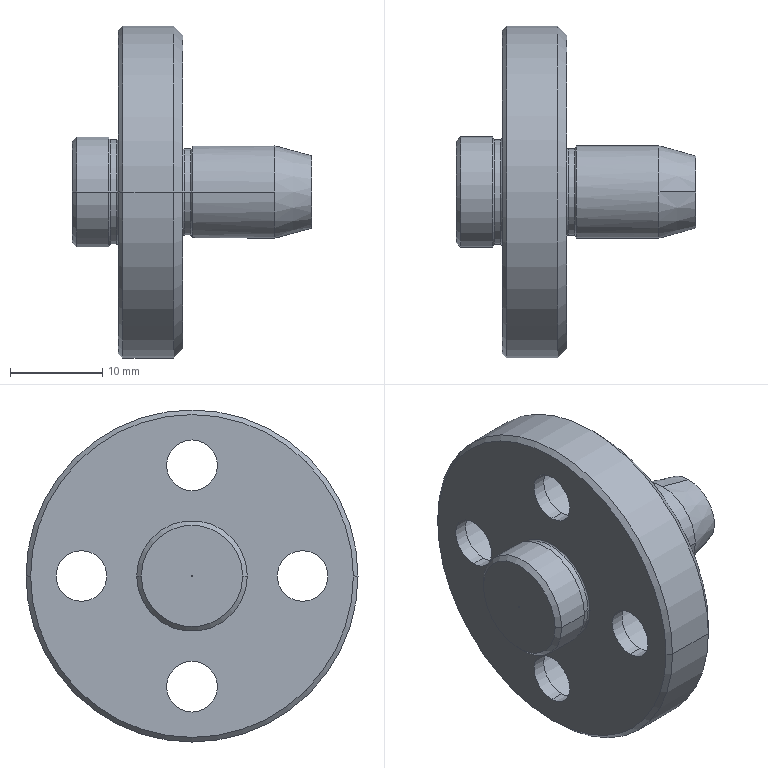Part | STEP file | MISUMI_MASAA12-P10.00-B10.0-T7.0_Locating pin | 1 solid | 56 faces | box 26 x 36 x 36 mm | volume 6932 mm3 | cylinder 26 | cone 12 | plane 10 | torus 8 | commonest cylinder face diameters 5.5 x8 9.5 x8 9.4 x2 10 x2 11.4 x2 12 x2
STEP:
#1=CARTESIAN_POINT('',(25.9,0.,0.));
#2=VERTEX_POINT('',#1);
#3=CARTESIAN_POINT('',(26.,0.,-0.1));
#4=VERTEX_POINT('',#3);
#5=CARTESIAN_POINT('',(26.,0.,-0.1));
#6=DIRECTION('',(0.7071,0.,-0.7071));
#7=VECTOR('',#6,1000.);
#8=LINE('',#5,#7);
#9=EDGE_CURVE('',#2,#4,#8,.T.);
#10=ORIENTED_EDGE('',*,*,#9,.F.);
#11=CARTESIAN_POINT('',(26.,0.,0.1));
#12=VERTEX_POINT('',#11);
#13=CARTESIAN_POINT('',(26.,0.,0.1));
#14=DIRECTION('',(0.7071,0.,0.7071));
#15=VECTOR('',#14,1000.);
#16=LINE('',#13,#15);
#17=EDGE_CURVE('',#2,#12,#16,.T.);
#18=ORIENTED_EDGE('',*,*,#17,.T.);
#19=CARTESIAN_POINT('',(26.,0.,0.));
#20=DIRECTION('',(-1.,0.,0.));
#21=DIRECTION('',(0.,0.,1.));
#22=AXIS2_PLACEMENT_3D('',#19,#20,#21);
#23=CIRCLE('',#22,0.1);
#24=EDGE_CURVE('',#4,#12,#23,.T.);
#25=ORIENTED_EDGE('',*,*,#24,.F.);
#26=EDGE_LOOP('',(#10,#18,#25));
#27=FACE_OUTER_BOUND('',#26,.T.);
#28=CARTESIAN_POINT('',(26.,0.,0.));
#29=DIRECTION('',(1.,0.,0.));
#30=DIRECTION('',(0.,0.,-1.));
#31=AXIS2_PLACEMENT_3D('',#28,#29,#30);
#32=CONICAL_SURFACE('',#31,0.1,0.7854);
#33=ADVANCED_FACE('',(#27),#32,.F.);
#34=CARTESIAN_POINT('',(26.,0.,3.928));
#35=VERTEX_POINT('',#34);
#36=CARTESIAN_POINT('',(26.,0.,-3.928));
#37=VERTEX_POINT('',#36);
#38=CARTESIAN_POINT('',(26.,0.,0.));
#39=DIRECTION('',(-1.,0.,0.));
#40=DIRECTION('',(0.,0.,1.));
#41=AXIS2_PLACEMENT_3D('',#38,#39,#40);
#42=CIRCLE('',#41,3.928);
#43=EDGE_CURVE('',#35,#37,#42,.T.);
#44=ORIENTED_EDGE('',*,*,#43,.T.);
#45=CARTESIAN_POINT('',(22.,0.,-5.));
#46=VERTEX_POINT('',#45);
#47=CARTESIAN_POINT('',(26.,0.,-3.928));
#48=DIRECTION('',(-0.9659,0.,-0.2588));
#49=VECTOR('',#48,1000.);
#50=LINE('',#47,#49);
#51=EDGE_CURVE('',#37,#46,#50,.T.);
#52=ORIENTED_EDGE('',*,*,#51,.T.);
#53=CARTESIAN_POINT('',(22.,5.,0.));
#54=VERTEX_POINT('',#53);
#55=CARTESIAN_POINT('',(22.,0.,0.));
#56=DIRECTION('',(-1.,0.,0.));
#57=DIRECTION('',(0.,0.,1.));
#58=AXIS2_PLACEMENT_3D('',#55,#56,#57);
#59=CIRCLE('',#58,5.);
#60=EDGE_CURVE('',#54,#46,#59,.T.);
#61=ORIENTED_EDGE('',*,*,#60,.F.);
#62=CARTESIAN_POINT('',(22.,0.,5.));
#63=VERTEX_POINT('',#62);
#64=CARTESIAN_POINT('',(22.,0.,0.));
#65=DIRECTION('',(-1.,0.,0.));
#66=DIRECTION('',(0.,0.,1.));
#67=AXIS2_PLACEMENT_3D('',#64,#65,#66);
#68=CIRCLE('',#67,5.);
#69=EDGE_CURVE('',#63,#54,#68,.T.);
#70=ORIENTED_EDGE('',*,*,#69,.F.);
#71=CARTESIAN_POINT('',(26.,0.,3.928));
#72=DIRECTION('',(-0.9659,0.,0.2588));
#73=VECTOR('',#72,1000.);
#74=LINE('',#71,#73);
#75=EDGE_CURVE('',#35,#63,#74,.T.);
#76=ORIENTED_EDGE('',*,*,#75,.F.);
#77=EDGE_LOOP('',(#44,#52,#61,#70,#76));
#78=FACE_OUTER_BOUND('',#77,.T.);
#79=CARTESIAN_POINT('',(26.,0.,0.));
#80=DIRECTION('',(-1.,0.,0.));
#81=DIRECTION('',(0.,0.,1.));
#82=AXIS2_PLACEMENT_3D('',#79,#80,#81);
#83=CONICAL_SURFACE('',#82,3.928,0.2618);
#84=ADVANCED_FACE('',(#78),#83,.T.);
#85=CARTESIAN_POINT('',(12.,17.,0.));
#86=VERTEX_POINT('',#85);
#87=CARTESIAN_POINT('',(12.,-17.,0.));
#88=VERTEX_POINT('',#87);
#89=CARTESIAN_POINT('',(12.,0.,0.));
#90=DIRECTION('',(1.,0.,0.));
#91=DIRECTION('',(0.,-1.,0.));
#92=AXIS2_PLACEMENT_3D('',#89,#90,#91);
#93=CIRCLE('',#92,17.);
#94=EDGE_CURVE('',#86,#88,#93,.T.);
#95=ORIENTED_EDGE('',*,*,#94,.F.);
#96=CARTESIAN_POINT('',(11.,18.,0.));
#97=VERTEX_POINT('',#96);
#98=CARTESIAN_POINT('',(11.,18.,0.));
#99=DIRECTION('',(-0.7071,0.7071,0.));
#100=VECTOR('',#99,1000.);
#101=LINE('',#98,#100);
#102=EDGE_CURVE('',#86,#97,#101,.T.);
#103=ORIENTED_EDGE('',*,*,#102,.T.);
#104=CARTESIAN_POINT('',(11.,-18.,0.));
#105=VERTEX_POINT('',#104);
#106=CARTESIAN_POINT('',(11.,0.,0.));
#107=DIRECTION('',(-1.,0.,0.));
#108=DIRECTION('',(0.,-1.,0.));
#109=AXIS2_PLACEMENT_3D('',#106,#107,#108);
#110=CIRCLE('',#109,18.);
#111=EDGE_CURVE('',#105,#97,#110,.T.);
#112=ORIENTED_EDGE('',*,*,#111,.F.);
#113=CARTESIAN_POINT('',(11.,-18.,0.));
#114=DIRECTION('',(-0.7071,-0.7071,0.));
#115=VECTOR('',#114,1000.);
#116=LINE('',#113,#115);
#117=EDGE_CURVE('',#88,#105,#116,.T.);
#118=ORIENTED_EDGE('',*,*,#117,.F.);
#119=EDGE_LOOP('',(#95,#103,#112,#118));
#120=FACE_OUTER_BOUND('',#119,.T.);
#121=CARTESIAN_POINT('',(11.,0.,0.));
#122=DIRECTION('',(-1.,0.,0.));
#123=DIRECTION('',(0.,-1.,0.));
#124=AXIS2_PLACEMENT_3D('',#121,#122,#123);
#125=CONICAL_SURFACE('',#124,18.,0.7854);
#126=ADVANCED_FACE('',(#120),#125,.T.);
#127=CARTESIAN_POINT('',(5.,-17.5,0.));
#128=VERTEX_POINT('',#127);
#129=CARTESIAN_POINT('',(5.,17.5,0.));
#130=VERTEX_POINT('',#129);
#131=CARTESIAN_POINT('',(5.,0.,0.));
#132=DIRECTION('',(-1.,0.,0.));
#133=DIRECTION('',(0.,1.,0.));
#134=AXIS2_PLACEMENT_3D('',#131,#132,#133);
#135=CIRCLE('',#134,17.5);
#136=EDGE_CURVE('',#128,#130,#135,.T.);
#137=ORIENTED_EDGE('',*,*,#136,.F.);
#138=CARTESIAN_POINT('',(5.5,-18.,0.));
#139=VERTEX_POINT('',#138);
#140=CARTESIAN_POINT('',(5.,-17.5,0.));
#141=DIRECTION('',(0.7071,-0.7071,0.));
#142=VECTOR('',#141,1000.);
#143=LINE('',#140,#142);
#144=EDGE_CURVE('',#128,#139,#143,.T.);
#145=ORIENTED_EDGE('',*,*,#144,.T.);
#146=CARTESIAN_POINT('',(5.5,18.,0.));
#147=VERTEX_POINT('',#146);
#148=CARTESIAN_POINT('',(5.5,0.,0.));
#149=DIRECTION('',(1.,0.,0.));
#150=DIRECTION('',(0.,1.,0.));
#151=AXIS2_PLACEMENT_3D('',#148,#149,#150);
#152=CIRCLE('',#151,18.);
#153=EDGE_CURVE('',#147,#139,#152,.T.);
#154=ORIENTED_EDGE('',*,*,#153,.F.);
#155=CARTESIAN_POINT('',(5.,17.5,0.));
#156=DIRECTION('',(0.7071,0.7071,0.));
#157=VECTOR('',#156,1000.);
#158=LINE('',#155,#157);
#159=EDGE_CURVE('',#130,#147,#158,.T.);
#160=ORIENTED_EDGE('',*,*,#159,.F.);
#161=EDGE_LOOP('',(#137,#145,#154,#160));
#162=FACE_OUTER_BOUND('',#161,.T.);
#163=CARTESIAN_POINT('',(5.,0.,0.));
#164=DIRECTION('',(1.,0.,0.));
#165=DIRECTION('',(0.,1.,0.));
#166=AXIS2_PLACEMENT_3D('',#163,#164,#165);
#167=CONICAL_SURFACE('',#166,17.5,0.7854);
#168=ADVANCED_FACE('',(#162),#167,.T.);
#169=CARTESIAN_POINT('',(12.,4.85,0.));
#170=VERTEX_POINT('',#169);
#171=CARTESIAN_POINT('',(12.,-4.85,0.));
#172=VERTEX_POINT('',#171);
#173=CARTESIAN_POINT('',(12.,0.,0.));
#174=DIRECTION('',(-1.,0.,0.));
#175=DIRECTION('',(0.,-1.,0.));
#176=AXIS2_PLACEMENT_3D('',#173,#174,#175);
#177=CIRCLE('',#176,4.85);
#178=EDGE_CURVE('',#170,#172,#177,.T.);
#179=ORIENTED_EDGE('',*,*,#178,.F.);
#180=CARTESIAN_POINT('',(12.15,4.7,0.));
#181=VERTEX_POINT('',#180);
#182=CARTESIAN_POINT('',(12.15,4.85,0.));
#183=DIRECTION('',(0.,0.,1.));
#184=DIRECTION('',(0.,-1.,0.));
#185=AXIS2_PLACEMENT_3D('',#182,#183,#184);
#186=CIRCLE('',#185,0.15);
#187=EDGE_CURVE('',#170,#181,#186,.T.);
#188=ORIENTED_EDGE('',*,*,#187,.T.);
#189=CARTESIAN_POINT('',(12.15,-4.7,0.));
#190=VERTEX_POINT('',#189);
#191=CARTESIAN_POINT('',(12.15,0.,0.));
#192=DIRECTION('',(1.,0.,0.));
#193=DIRECTION('',(0.,-1.,0.));
#194=AXIS2_PLACEMENT_3D('',#191,#192,#193);
#195=CIRCLE('',#194,4.7);
#196=EDGE_CURVE('',#190,#181,#195,.T.);
#197=ORIENTED_EDGE('',*,*,#196,.F.);
#198=CARTESIAN_POINT('',(12.15,-4.85,0.));
#199=DIRECTION('',(0.,0.,-1.));
#200=DIRECTION('',(-1.,0.,0.));
#201=AXIS2_PLACEMENT_3D('',#198,#199,#200);
#202=CIRCLE('',#201,0.15);
#203=EDGE_CURVE('',#172,#190,#202,.T.);
#204=ORIENTED_EDGE('',*,*,#203,.F.);
#205=EDGE_LOOP('',(#179,#188,#197,#204));
#206=FACE_OUTER_BOUND('',#205,.T.);
#207=CARTESIAN_POINT('',(12.15,0.,0.));
#208=DIRECTION('',(-1.,0.,0.));
#209=DIRECTION('',(0.,-1.,0.));
#210=AXIS2_PLACEMENT_3D('',#207,#208,#209);
#211=TOROIDAL_SURFACE('',#210,4.85,0.15);
#212=ADVANCED_FACE('',(#206),#211,.F.);
#213=CARTESIAN_POINT('',(13.,-4.85,0.));
#214=VERTEX_POINT('',#213);
#215=CARTESIAN_POINT('',(13.,4.85,0.));
#216=VERTEX_POINT('',#215);
#217=CARTESIAN_POINT('',(13.,0.,0.));
#218=DIRECTION('',(1.,0.,0.));
#219=DIRECTION('',(0.,1.,0.));
#220=AXIS2_PLACEMENT_3D('',#217,#218,#219);
#221=CIRCLE('',#220,4.85);
#222=EDGE_CURVE('',#214,#216,#221,.T.);
#223=ORIENTED_EDGE('',*,*,#222,.F.);
#224=CARTESIAN_POINT('',(12.85,-4.7,0.));
#225=VERTEX_POINT('',#224);
#226=CARTESIAN_POINT('',(12.85,-4.85,0.));
#227=DIRECTION('',(0.,0.,1.));
#228=DIRECTION('',(0.,-1.,0.));
#229=AXIS2_PLACEMENT_3D('',#226,#227,#228);
#230=CIRCLE('',#229,0.15);
#231=EDGE_CURVE('',#214,#225,#230,.T.);
#232=ORIENTED_EDGE('',*,*,#231,.T.);
#233=CARTESIAN_POINT('',(12.85,4.7,0.));
#234=VERTEX_POINT('',#233);
#235=CARTESIAN_POINT('',(12.85,0.,0.));
#236=DIRECTION('',(-1.,0.,0.));
#237=DIRECTION('',(0.,1.,0.));
#238=AXIS2_PLACEMENT_3D('',#235,#236,#237);
#239=CIRCLE('',#238,4.7);
#240=EDGE_CURVE('',#234,#225,#239,.T.);
#241=ORIENTED_EDGE('',*,*,#240,.F.);
#242=CARTESIAN_POINT('',(12.85,4.85,0.));
#243=DIRECTION('',(0.,0.,-1.));
#244=DIRECTION('',(-1.,0.,0.));
#245=AXIS2_PLACEMENT_3D('',#242,#243,#244);
#246=CIRCLE('',#245,0.15);
#247=EDGE_CURVE('',#216,#234,#246,.T.);
#248=ORIENTED_EDGE('',*,*,#247,.F.);
#249=EDGE_LOOP('',(#223,#232,#241,#248));
#250=FACE_OUTER_BOUND('',#249,.T.);
#251=CARTESIAN_POINT('',(12.85,0.,0.));
#252=DIRECTION('',(1.,0.,0.));
#253=DIRECTION('',(0.,1.,0.));
#254=AXIS2_PLACEMENT_3D('',#251,#252,#253);
#255=TOROIDAL_SURFACE('',#254,4.85,0.15);
#256=ADVANCED_FACE('',(#250),#255,.F.);
#257=CARTESIAN_POINT('',(5.,-5.85,0.));
#258=VERTEX_POINT('',#257);
#259=CARTESIAN_POINT('',(5.,5.85,0.));
#260=VERTEX_POINT('',#259);
#261=CARTESIAN_POINT('',(5.,0.,0.));
#262=DIRECTION('',(1.,0.,0.));
#263=DIRECTION('',(0.,1.,0.));
#264=AXIS2_PLACEMENT_3D('',#261,#262,#263);
#265=CIRCLE('',#264,5.85);
#266=EDGE_CURVE('',#258,#260,#265,.T.);
#267=ORIENTED_EDGE('',*,*,#266,.F.);
#268=CARTESIAN_POINT('',(4.85,-5.7,0.));
#269=VERTEX_POINT('',#268);
#270=CARTESIAN_POINT('',(4.85,-5.85,0.));
#271=DIRECTION('',(0.,0.,1.));
#272=DIRECTION('',(0.,-1.,0.));
#273=AXIS2_PLACEMENT_3D('',#270,#271,#272);
#274=CIRCLE('',#273,0.15);
#275=EDGE_CURVE('',#258,#269,#274,.T.);
#276=ORIENTED_EDGE('',*,*,#275,.T.);
#277=CARTESIAN_POINT('',(4.85,5.7,0.));
#278=VERTEX_POINT('',#277);
#279=CARTESIAN_POINT('',(4.85,0.,0.));
#280=DIRECTION('',(-1.,0.,0.));
#281=DIRECTION('',(0.,1.,0.));
#282=AXIS2_PLACEMENT_3D('',#279,#280,#281);
#283=CIRCLE('',#282,5.7);
#284=EDGE_CURVE('',#278,#269,#283,.T.);
#285=ORIENTED_EDGE('',*,*,#284,.F.);
#286=CARTESIAN_POINT('',(4.85,5.85,0.));
#287=DIRECTION('',(0.,0.,-1.));
#288=DIRECTION('',(-1.,0.,0.));
#289=AXIS2_PLACEMENT_3D('',#286,#287,#288);
#290=CIRCLE('',#289,0.15);
#291=EDGE_CURVE('',#260,#278,#290,.T.);
#292=ORIENTED_EDGE('',*,*,#291,.F.);
#293=EDGE_LOOP('',(#267,#276,#285,#292));
#294=FACE_OUTER_BOUND('',#293,.T.);
#295=CARTESIAN_POINT('',(4.85,0.,0.));
#296=DIRECTION('',(1.,0.,0.));
#297=DIRECTION('',(0.,1.,0.));
#298=AXIS2_PLACEMENT_3D('',#295,#296,#297);
#299=TOROIDAL_SURFACE('',#298,5.85,0.15);
#300=ADVANCED_FACE('',(#294),#299,.F.);
#301=CARTESIAN_POINT('',(4.,5.85,0.));
#302=VERTEX_POINT('',#301);
#303=CARTESIAN_POINT('',(4.,-5.85,0.));
#304=VERTEX_POINT('',#303);
#305=CARTESIAN_POINT('',(4.,0.,0.));
#306=DIRECTION('',(-1.,0.,0.));
#307=DIRECTION('',(0.,-1.,0.));
#308=AXIS2_PLACEMENT_3D('',#305,#306,#307);
#309=CIRCLE('',#308,5.85);
#310=EDGE_CURVE('',#302,#304,#309,.T.);
#311=ORIENTED_EDGE('',*,*,#310,.F.);
#312=CARTESIAN_POINT('',(4.15,5.7,0.));
#313=VERTEX_POINT('',#312);
#314=CARTESIAN_POINT('',(4.15,5.85,0.));
#315=DIRECTION('',(0.,0.,1.));
#316=DIRECTION('',(0.,-1.,0.));
#317=AXIS2_PLACEMENT_3D('',#314,#315,#316);
#318=CIRCLE('',#317,0.15);
#319=EDGE_CURVE('',#302,#313,#318,.T.);
#320=ORIENTED_EDGE('',*,*,#319,.T.);
#321=CARTESIAN_POINT('',(4.15,-5.7,0.));
#322=VERTEX_POINT('',#321);
#323=CARTESIAN_POINT('',(4.15,0.,0.));
#324=DIRECTION('',(1.,0.,0.));
#325=DIRECTION('',(0.,-1.,0.));
#326=AXIS2_PLACEMENT_3D('',#323,#324,#325);
#327=CIRCLE('',#326,5.7);
#328=EDGE_CURVE('',#322,#313,#327,.T.);
#329=ORIENTED_EDGE('',*,*,#328,.F.);
#330=CARTESIAN_POINT('',(4.15,-5.85,0.));
#331=DIRECTION('',(0.,0.,-1.));
#332=DIRECTION('',(-1.,0.,0.));
#333=AXIS2_PLACEMENT_3D('',#330,#331,#332);
#334=CIRCLE('',#333,0.15);
#335=EDGE_CURVE('',#304,#322,#334,.T.);
#336=ORIENTED_EDGE('',*,*,#335,.F.);
#337=EDGE_LOOP('',(#311,#320,#329,#336));
#338=FACE_OUTER_BOUND('',#337,.T.);
#339=CARTESIAN_POINT('',(4.15,0.,0.));
#340=DIRECTION('',(-1.,0.,0.));
#341=DIRECTION('',(0.,-1.,0.));
#342=AXIS2_PLACEMENT_3D('',#339,#340,#341);
#343=TOROIDAL_SURFACE('',#342,5.85,0.15);
#344=ADVANCED_FACE('',(#338),#343,.F.);
#345=CARTESIAN_POINT('',(0.,-5.5,0.));
#346=VERTEX_POINT('',#345);
#347=CARTESIAN_POINT('',(0.,5.5,0.));
#348=VERTEX_POINT('',#347);
#349=CARTESIAN_POINT('',(0.,0.,0.));
#350=DIRECTION('',(-1.,0.,0.));
#351=DIRECTION('',(0.,1.,0.));
#352=AXIS2_PLACEMENT_3D('',#349,#350,#351);
#353=CIRCLE('',#352,5.5);
#354=EDGE_CURVE('',#346,#348,#353,.T.);
#355=ORIENTED_EDGE('',*,*,#354,.F.);
#356=CARTESIAN_POINT('',(0.5,-6.,0.));
#357=VERTEX_POINT('',#356);
#358=CARTESIAN_POINT('',(0.,-5.5,0.));
#359=DIRECTION('',(0.7071,-0.7071,0.));
#360=VECTOR('',#359,1000.);
#361=LINE('',#358,#360);
#362=EDGE_CURVE('',#346,#357,#361,.T.);
#363=ORIENTED_EDGE('',*,*,#362,.T.);
#364=CARTESIAN_POINT('',(0.5,6.,0.));
#365=VERTEX_POINT('',#364);
#366=CARTESIAN_POINT('',(0.5,0.,0.));
#367=DIRECTION('',(1.,0.,0.));
#368=DIRECTION('',(0.,1.,0.));
#369=AXIS2_PLACEMENT_3D('',#366,#367,#368);
#370=CIRCLE('',#369,6.);
#371=EDGE_CURVE('',#365,#357,#370,.T.);
#372=ORIENTED_EDGE('',*,*,#371,.F.);
#373=CARTESIAN_POINT('',(0.,5.5,0.));
#374=DIRECTION('',(0.7071,0.7071,0.));
#375=VECTOR('',#374,1000.);
#376=LINE('',#373,#375);
#377=EDGE_CURVE('',#348,#365,#376,.T.);
#378=ORIENTED_EDGE('',*,*,#377,.F.);
#379=EDGE_LOOP('',(#355,#363,#372,#378));
#380=FACE_OUTER_BOUND('',#379,.T.);
#381=CARTESIAN_POINT('',(0.,0.,0.));
#382=DIRECTION('',(1.,0.,0.));
#383=DIRECTION('',(0.,1.,0.));
#384=AXIS2_PLACEMENT_3D('',#381,#382,#383);
#385=CONICAL_SURFACE('',#384,5.5,0.7854);
#386=ADVANCED_FACE('',(#380),#385,.T.);
#387=CARTESIAN_POINT('',(6.5,12.,4.75));
#388=VERTEX_POINT('',#387);
#389=CARTESIAN_POINT('',(6.5,12.,-4.75));
#390=VERTEX_POINT('',#389);
#391=CARTESIAN_POINT('',(6.5,12.,0.));
#392=DIRECTION('',(1.,0.,0.));
#393=DIRECTION('',(0.,0.,-1.));
#394=AXIS2_PLACEMENT_3D('',#391,#392,#393);
#395=CIRCLE('',#394,4.75);
#396=EDGE_CURVE('',#388,#390,#395,.T.);
#397=ORIENTED_EDGE('',*,*,#396,.F.);
#398=CARTESIAN_POINT('',(12.,12.,4.75));
#399=VERTEX_POINT('',#398);
#400=CARTESIAN_POINT('',(12.,12.,4.75));
#401=DIRECTION('',(1.,0.,0.));
#402=VECTOR('',#401,1000.);
#403=LINE('',#400,#402);
#404=EDGE_CURVE('',#388,#399,#403,.T.);
#405=ORIENTED_EDGE('',*,*,#404,.T.);
#406=CARTESIAN_POINT('',(12.,12.,-4.75));
#407=VERTEX_POINT('',#406);
#408=CARTESIAN_POINT('',(12.,12.,0.));
#409=DIRECTION('',(1.,0.,0.));
#410=DIRECTION('',(0.,0.,-1.));
#411=AXIS2_PLACEMENT_3D('',#408,#409,#410);
#412=CIRCLE('',#411,4.75);
#413=EDGE_CURVE('',#399,#407,#412,.T.);
#414=ORIENTED_EDGE('',*,*,#413,.T.);
#415=CARTESIAN_POINT('',(12.,12.,-4.75));
#416=DIRECTION('',(1.,0.,0.));
#417=VECTOR('',#416,1000.);
#418=LINE('',#415,#417);
#419=EDGE_CURVE('',#390,#407,#418,.T.);
#420=ORIENTED_EDGE('',*,*,#419,.F.);
#421=EDGE_LOOP('',(#397,#405,#414,#420));
#422=FACE_OUTER_BOUND('',#421,.T.);
#423=CARTESIAN_POINT('',(12.,12.,0.));
#424=DIRECTION('',(1.,0.,0.));
#425=DIRECTION('',(0.,0.,-1.));
#426=AXIS2_PLACEMENT_3D('',#423,#424,#425);
#427=CYLINDRICAL_SURFACE('',#426,4.75);
#428=ADVANCED_FACE('',(#422),#427,.F.);
#429=CARTESIAN_POINT('',(5.,12.,2.75));
#430=VERTEX_POINT('',#429);
#431=CARTESIAN_POINT('',(5.,12.,-2.75));
#432=VERTEX_POINT('',#431);
#433=CARTESIAN_POINT('',(5.,12.,0.));
#434=DIRECTION('',(1.,0.,0.));
#435=DIRECTION('',(0.,1.,0.));
#436=AXIS2_PLACEMENT_3D('',#433,#434,#435);
#437=CIRCLE('',#436,2.75);
#438=EDGE_CURVE('',#430,#432,#437,.T.);
#439=ORIENTED_EDGE('',*,*,#438,.F.);
#440=CARTESIAN_POINT('',(6.5,12.,2.75));
#441=VERTEX_POINT('',#440);
#442=CARTESIAN_POINT('',(12.,12.,2.75));
#443=DIRECTION('',(1.,0.,0.));
#444=VECTOR('',#443,1000.);
#445=LINE('',#442,#444);
#446=EDGE_CURVE('',#430,#441,#445,.T.);
#447=ORIENTED_EDGE('',*,*,#446,.T.);
#448=CARTESIAN_POINT('',(6.5,12.,-2.75));
#449=VERTEX_POINT('',#448);
#450=CARTESIAN_POINT('',(6.5,12.,0.));
#451=DIRECTION('',(1.,0.,0.));
#452=DIRECTION('',(0.,0.,-1.));
#453=AXIS2_PLACEMENT_3D('',#450,#451,#452);
#454=CIRCLE('',#453,2.75);
#455=EDGE_CURVE('',#441,#449,#454,.T.);
#456=ORIENTED_EDGE('',*,*,#455,.T.);
#457=CARTESIAN_POINT('',(12.,12.,-2.75));
#458=DIRECTION('',(1.,0.,0.));
#459=VECTOR('',#458,1000.);
#460=LINE('',#457,#459);
#461=EDGE_CURVE('',#432,#449,#460,.T.);
#462=ORIENTED_EDGE('',*,*,#461,.F.);
#463=EDGE_LOOP('',(#439,#447,#456,#462));
#464=FACE_OUTER_BOUND('',#463,.T.);
#465=CARTESIAN_POINT('',(12.,12.,0.));
#466=DIRECTION('',(1.,0.,0.));
#467=DIRECTION('',(0.,0.,-1.));
#468=AXIS2_PLACEMENT_3D('',#465,#466,#467);
#469=CYLINDRICAL_SURFACE('',#468,2.75);
#470=ADVANCED_FACE('',(#464),#469,.F.);
#471=CARTESIAN_POINT('',(6.5,0.,16.75));
#472=VERTEX_POINT('',#471);
#473=CARTESIAN_POINT('',(6.5,0.,7.25));
#474=VERTEX_POINT('',#473);
#475=CARTESIAN_POINT('',(6.5,0.,12.));
#476=DIRECTION('',(1.,0.,0.));
#477=DIRECTION('',(0.,0.,-1.));
#478=AXIS2_PLACEMENT_3D('',#475,#476,#477);
#479=CIRCLE('',#478,4.75);
#480=EDGE_CURVE('',#472,#474,#479,.T.);
#481=ORIENTED_EDGE('',*,*,#480,.F.);
#482=CARTESIAN_POINT('',(12.,0.,16.75));
#483=VERTEX_POINT('',#482);
#484=CARTESIAN_POINT('',(12.,0.,16.75));
#485=DIRECTION('',(1.,0.,0.));
#486=VECTOR('',#485,1000.);
#487=LINE('',#484,#486);
#488=EDGE_CURVE('',#472,#483,#487,.T.);
#489=ORIENTED_EDGE('',*,*,#488,.T.);
#490=CARTESIAN_POINT('',(12.,0.,7.25));
#491=VERTEX_POINT('',#490);
#492=CARTESIAN_POINT('',(12.,0.,12.));
#493=DIRECTION('',(1.,0.,0.));
#494=DIRECTION('',(0.,0.,-1.));
#495=AXIS2_PLACEMENT_3D('',#492,#493,#494);
#496=CIRCLE('',#495,4.75);
#497=EDGE_CURVE('',#483,#491,#496,.T.);
#498=ORIENTED_EDGE('',*,*,#497,.T.);
#499=CARTESIAN_POINT('',(12.,0.,7.25));
#500=DIRECTION('',(1.,0.,0.));
#501=VECTOR('',#500,1000.);
#502=LINE('',#499,#501);
#503=EDGE_CURVE('',#474,#491,#502,.T.);
#504=ORIENTED_EDGE('',*,*,#503,.F.);
#505=EDGE_LOOP('',(#481,#489,#498,#504));
#506=FACE_OUTER_BOUND('',#505,.T.);
#507=CARTESIAN_POINT('',(12.,0.,12.));
#508=DIRECTION('',(1.,0.,0.));
#509=DIRECTION('',(0.,0.,-1.));
#510=AXIS2_PLACEMENT_3D('',#507,#508,#509);
#511=CYLINDRICAL_SURFACE('',#510,4.75);
#512=ADVANCED_FACE('',(#506),#511,.F.);
#513=CARTESIAN_POINT('',(5.,0.,14.75));
#514=VERTEX_POINT('',#513);
#515=CARTESIAN_POINT('',(5.,0.,9.25));
#516=VERTEX_POINT('',#515);
#517=CARTESIAN_POINT('',(5.,0.,12.));
#518=DIRECTION('',(1.,0.,0.));
#519=DIRECTION('',(0.,1.,0.));
#520=AXIS2_PLACEMENT_3D('',#517,#518,#519);
#521=CIRCLE('',#520,2.75);
#522=EDGE_CURVE('',#514,#516,#521,.T.);
#523=ORIENTED_EDGE('',*,*,#522,.F.);
#524=CARTESIAN_POINT('',(6.5,0.,14.75));
#525=VERTEX_POINT('',#524);
#526=CARTESIAN_POINT('',(12.,0.,14.75));
#527=DIRECTION('',(1.,0.,0.));
#528=VECTOR('',#527,1000.);
#529=LINE('',#526,#528);
#530=EDGE_CURVE('',#514,#525,#529,.T.);
#531=ORIENTED_EDGE('',*,*,#530,.T.);
#532=CARTESIAN_POINT('',(6.5,0.,9.25));
#533=VERTEX_POINT('',#532);
#534=CARTESIAN_POINT('',(6.5,0.,12.));
#535=DIRECTION('',(1.,0.,0.));
#536=DIRECTION('',(0.,0.,-1.));
#537=AXIS2_PLACEMENT_3D('',#534,#535,#536);
#538=CIRCLE('',#537,2.75);
#539=EDGE_CURVE('',#525,#533,#538,.T.);
#540=ORIENTED_EDGE('',*,*,#539,.T.);
#541=CARTESIAN_POINT('',(12.,0.,9.25));
#542=DIRECTION('',(1.,0.,0.));
#543=VECTOR('',#542,1000.);
#544=LINE('',#541,#543);
#545=EDGE_CURVE('',#516,#533,#544,.T.);
#546=ORIENTED_EDGE('',*,*,#545,.F.);
#547=EDGE_LOOP('',(#523,#531,#540,#546));
#548=FACE_OUTER_BOUND('',#547,.T.);
#549=CARTESIAN_POINT('',(12.,0.,12.));
#550=DIRECTION('',(1.,0.,0.));
#551=DIRECTION('',(0.,0.,-1.));
#552=AXIS2_PLACEMENT_3D('',#549,#550,#551);
#553=CYLINDRICAL_SURFACE('',#552,2.75);
#554=ADVANCED_FACE('',(#548),#553,.F.);
#555=CARTESIAN_POINT('',(6.5,-12.,4.75));
#556=VERTEX_POINT('',#555);
#557=CARTESIAN_POINT('',(6.5,-12.,-4.75));
#558=VERTEX_POINT('',#557);
#559=CARTESIAN_POINT('',(6.5,-12.,0.));
#560=DIRECTION('',(1.,0.,0.));
#561=DIRECTION('',(0.,0.,-1.));
#562=AXIS2_PLACEMENT_3D('',#559,#560,#561);
#563=CIRCLE('',#562,4.75);
#564=EDGE_CURVE('',#556,#558,#563,.T.);
#565=ORIENTED_EDGE('',*,*,#564,.F.);
#566=CARTESIAN_POINT('',(12.,-12.,4.75));
#567=VERTEX_POINT('',#566);
#568=CARTESIAN_POINT('',(12.,-12.,4.75));
#569=DIRECTION('',(1.,0.,0.));
#570=VECTOR('',#569,1000.);
#571=LINE('',#568,#570);
#572=EDGE_CURVE('',#556,#567,#571,.T.);
#573=ORIENTED_EDGE('',*,*,#572,.T.);
#574=CARTESIAN_POINT('',(12.,-12.,-4.75));
#575=VERTEX_POINT('',#574);
#576=CARTESIAN_POINT('',(12.,-12.,0.));
#577=DIRECTION('',(1.,0.,0.));
#578=DIRECTION('',(0.,0.,-1.));
#579=AXIS2_PLACEMENT_3D('',#576,#577,#578);
#580=CIRCLE('',#579,4.75);
#581=EDGE_CURVE('',#567,#575,#580,.T.);
#582=ORIENTED_EDGE('',*,*,#581,.T.);
#583=CARTESIAN_POINT('',(12.,-12.,-4.75));
#584=DIRECTION('',(1.,0.,0.));
#585=VECTOR('',#584,1000.);
#586=LINE('',#583,#585);
#587=EDGE_CURVE('',#558,#575,#586,.T.);
#588=ORIENTED_EDGE('',*,*,#587,.F.);
#589=EDGE_LOOP('',(#565,#573,#582,#588));
#590=FACE_OUTER_BOUND('',#589,.T.);
#591=CARTESIAN_POINT('',(12.,-12.,0.));
#592=DIRECTION('',(1.,0.,0.));
#593=DIRECTION('',(0.,0.,-1.));
#594=AXIS2_PLACEMENT_3D('',#591,#592,#593);
#595=CYLINDRICAL_SURFACE('',#594,4.75);
#596=ADVANCED_FACE('',(#590),#595,.F.);
#597=CARTESIAN_POINT('',(5.,-12.,2.75));
#598=VERTEX_POINT('',#597);
#599=CARTESIAN_POINT('',(5.,-12.,-2.75));
#600=VERTEX_POINT('',#599);
#601=CARTESIAN_POINT('',(5.,-12.,0.));
#602=DIRECTION('',(1.,0.,0.));
#603=DIRECTION('',(0.,1.,0.));
#604=AXIS2_PLACEMENT_3D('',#601,#602,#603);
#605=CIRCLE('',#604,2.75);
#606=EDGE_CURVE('',#598,#600,#605,.T.);
#607=ORIENTED_EDGE('',*,*,#606,.F.);
#608=CARTESIAN_POINT('',(6.5,-12.,2.75));
#609=VERTEX_POINT('',#608);
#610=CARTESIAN_POINT('',(12.,-12.,2.75));
#611=DIRECTION('',(1.,0.,0.));
#612=VECTOR('',#611,1000.);
#613=LINE('',#610,#612);
#614=EDGE_CURVE('',#598,#609,#613,.T.);
#615=ORIENTED_EDGE('',*,*,#614,.T.);
#616=CARTESIAN_POINT('',(6.5,-12.,-2.75));
#617=VERTEX_POINT('',#616);
#618=CARTESIAN_POINT('',(6.5,-12.,0.));
#619=DIRECTION('',(1.,0.,0.));
#620=DIRECTION('',(0.,0.,-1.));
#621=AXIS2_PLACEMENT_3D('',#618,#619,#620);
#622=CIRCLE('',#621,2.75);
#623=EDGE_CURVE('',#609,#617,#622,.T.);
#624=ORIENTED_EDGE('',*,*,#623,.T.);
#625=CARTESIAN_POINT('',(12.,-12.,-2.75));
#626=DIRECTION('',(1.,0.,0.));
#627=VECTOR('',#626,1000.);
#628=LINE('',#625,#627);
#629=EDGE_CURVE('',#600,#617,#628,.T.);
#630=ORIENTED_EDGE('',*,*,#629,.F.);
#631=EDGE_LOOP('',(#607,#615,#624,#630));
#632=FACE_OUTER_BOUND('',#631,.T.);
#633=CARTESIAN_POINT('',(12.,-12.,0.));
#634=DIRECTION('',(1.,0.,0.));
#635=DIRECTION('',(0.,0.,-1.));
#636=AXIS2_PLACEMENT_3D('',#633,#634,#635);
#637=CYLINDRICAL_SURFACE('',#636,2.75);
#638=ADVANCED_FACE('',(#632),#637,.F.);
#639=CARTESIAN_POINT('',(6.5,0.,-7.25));
#640=VERTEX_POINT('',#639);
#641=CARTESIAN_POINT('',(6.5,0.,-16.75));
#642=VERTEX_POINT('',#641);
#643=CARTESIAN_POINT('',(6.5,0.,-12.));
#644=DIRECTION('',(1.,0.,0.));
#645=DIRECTION('',(0.,0.,-1.));
#646=AXIS2_PLACEMENT_3D('',#643,#644,#645);
#647=CIRCLE('',#646,4.75);
#648=EDGE_CURVE('',#640,#642,#647,.T.);
#649=ORIENTED_EDGE('',*,*,#648,.F.);
#650=CARTESIAN_POINT('',(12.,0.,-7.25));
#651=VERTEX_POINT('',#650);
#652=CARTESIAN_POINT('',(12.,0.,-7.25));
#653=DIRECTION('',(1.,0.,0.));
#654=VECTOR('',#653,1000.);
#655=LINE('',#652,#654);
#656=EDGE_CURVE('',#640,#651,#655,.T.);
#657=ORIENTED_EDGE('',*,*,#656,.T.);
#658=CARTESIAN_POINT('',(12.,0.,-16.75));
#659=VERTEX_POINT('',#658);
#660=CARTESIAN_POINT('',(12.,0.,-12.));
#661=DIRECTION('',(1.,0.,0.));
#662=DIRECTION('',(0.,0.,-1.));
#663=AXIS2_PLACEMENT_3D('',#660,#661,#662);
#664=CIRCLE('',#663,4.75);
#665=EDGE_CURVE('',#651,#659,#664,.T.);
#666=ORIENTED_EDGE('',*,*,#665,.T.);
#667=CARTESIAN_POINT('',(12.,0.,-16.75));
#668=DIRECTION('',(1.,0.,0.));
#669=VECTOR('',#668,1000.);
#670=LINE('',#667,#669);
#671=EDGE_CURVE('',#642,#659,#670,.T.);
#672=ORIENTED_EDGE('',*,*,#671,.F.);
#673=EDGE_LOOP('',(#649,#657,#666,#672));
#674=FACE_OUTER_BOUND('',#673,.T.);
#675=CARTESIAN_POINT('',(12.,0.,-12.));
#676=DIRECTION('',(1.,0.,0.));
#677=DIRECTION('',(0.,0.,-1.));
#678=AXIS2_PLACEMENT_3D('',#675,#676,#677);
#679=CYLINDRICAL_SURFACE('',#678,4.75);
#680=ADVANCED_FACE('',(#674),#679,.F.);
#681=CARTESIAN_POINT('',(5.,0.,-9.25));
#682=VERTEX_POINT('',#681);
#683=CARTESIAN_POINT('',(5.,0.,-14.75));
#684=VERTEX_POINT('',#683);
#685=CARTESIAN_POINT('',(5.,0.,-12.));
#686=DIRECTION('',(1.,0.,0.));
#687=DIRECTION('',(0.,1.,0.));
#688=AXIS2_PLACEMENT_3D('',#685,#686,#687);
#689=CIRCLE('',#688,2.75);
#690=EDGE_CURVE('',#682,#684,#689,.T.);
#691=ORIENTED_EDGE('',*,*,#690,.F.);
#692=CARTESIAN_POINT('',(6.5,0.,-9.25));
#693=VERTEX_POINT('',#692);
#694=CARTESIAN_POINT('',(12.,0.,-9.25));
#695=DIRECTION('',(1.,0.,0.));
#696=VECTOR('',#695,1000.);
#697=LINE('',#694,#696);
#698=EDGE_CURVE('',#682,#693,#697,.T.);
#699=ORIENTED_EDGE('',*,*,#698,.T.);
#700=CARTESIAN_POINT('',(6.5,0.,-14.75));
#701=VERTEX_POINT('',#700);
#702=CARTESIAN_POINT('',(6.5,0.,-12.));
#703=DIRECTION('',(1.,0.,0.));
#704=DIRECTION('',(0.,0.,-1.));
#705=AXIS2_PLACEMENT_3D('',#702,#703,#704);
#706=CIRCLE('',#705,2.75);
#707=EDGE_CURVE('',#693,#701,#706,.T.);
#708=ORIENTED_EDGE('',*,*,#707,.T.);
#709=CARTESIAN_POINT('',(12.,0.,-14.75));
#710=DIRECTION('',(1.,0.,0.));
#711=VECTOR('',#710,1000.);
#712=LINE('',#709,#711);
#713=EDGE_CURVE('',#684,#701,#712,.T.);
#714=ORIENTED_EDGE('',*,*,#713,.F.);
#715=EDGE_LOOP('',(#691,#699,#708,#714));
#716=FACE_OUTER_BOUND('',#715,.T.);
#717=CARTESIAN_POINT('',(12.,0.,-12.));
#718=DIRECTION('',(1.,0.,0.));
#719=DIRECTION('',(0.,0.,-1.));
#720=AXIS2_PLACEMENT_3D('',#717,#718,#719);
#721=CYLINDRICAL_SURFACE('',#720,2.75);
#722=ADVANCED_FACE('',(#716),#721,.F.);
#723=CARTESIAN_POINT('',(0.1,0.,0.));
#724=VERTEX_POINT('',#723);
#725=CARTESIAN_POINT('',(0.,0.,0.1));
#726=VERTEX_POINT('',#725);
#727=CARTESIAN_POINT('',(0.1,0.,0.));
#728=DIRECTION('',(-0.7071,0.,0.7071));
#729=VECTOR('',#728,1000.);
#730=LINE('',#727,#729);
#731=EDGE_CURVE('',#724,#726,#730,.T.);
#732=ORIENTED_EDGE('',*,*,#731,.F.);
#733=CARTESIAN_POINT('',(0.,0.,-0.1));
#734=VERTEX_POINT('',#733);
#735=CARTESIAN_POINT('',(0.1,0.,0.));
#736=DIRECTION('',(-0.7071,0.,-0.7071));
#737=VECTOR('',#736,1000.);
#738=LINE('',#735,#737);
#739=EDGE_CURVE('',#724,#734,#738,.T.);
#740=ORIENTED_EDGE('',*,*,#739,.T.);
#741=CARTESIAN_POINT('',(0.,0.,0.));
#742=DIRECTION('',(-1.,0.,0.));
#743=DIRECTION('',(0.,0.,1.));
#744=AXIS2_PLACEMENT_3D('',#741,#742,#743);
#745=CIRCLE('',#744,0.1);
#746=EDGE_CURVE('',#734,#726,#745,.T.);
#747=ORIENTED_EDGE('',*,*,#746,.T.);
#748=EDGE_LOOP('',(#732,#740,#747));
#749=FACE_OUTER_BOUND('',#748,.T.);
#750=CARTESIAN_POINT('',(-999.9,0.,0.));
#751=DIRECTION('',(-1.,0.,0.));
#752=DIRECTION('',(0.,0.,1.));
#753=AXIS2_PLACEMENT_3D('',#750,#751,#752);
#754=CONICAL_SURFACE('',#753,1000.,0.7854);
#755=ADVANCED_FACE('',(#749),#754,.F.);
#756=CARTESIAN_POINT('',(22.,-5.,0.));
#757=VERTEX_POINT('',#756);
#758=CARTESIAN_POINT('',(22.,0.,0.));
#759=DIRECTION('',(-1.,0.,0.));
#760=DIRECTION('',(0.,0.,1.));
#761=AXIS2_PLACEMENT_3D('',#758,#759,#760);
#762=CIRCLE('',#761,5.);
#763=EDGE_CURVE('',#757,#63,#762,.T.);
#764=ORIENTED_EDGE('',*,*,#763,.T.);
#765=ORIENTED_EDGE('',*,*,#69,.T.);
#766=CARTESIAN_POINT('',(13.,5.,0.));
#767=VERTEX_POINT('',#766);
#768=CARTESIAN_POINT('',(0.,5.,0.));
#769=DIRECTION('',(-1.,0.,0.));
#770=VECTOR('',#769,1000.);
#771=LINE('',#768,#770);
#772=EDGE_CURVE('',#54,#767,#771,.T.);
#773=ORIENTED_EDGE('',*,*,#772,.T.);
#774=CARTESIAN_POINT('',(13.,-5.,0.));
#775=VERTEX_POINT('',#774);
#776=CARTESIAN_POINT('',(13.,0.,0.));
#777=DIRECTION('',(-1.,0.,0.));
#778=DIRECTION('',(0.,-1.,0.));
#779=AXIS2_PLACEMENT_3D('',#776,#777,#778);
#780=CIRCLE('',#779,5.);
#781=EDGE_CURVE('',#775,#767,#780,.T.);
#782=ORIENTED_EDGE('',*,*,#781,.F.);
#783=CARTESIAN_POINT('',(0.,-5.,0.));
#784=DIRECTION('',(-1.,0.,0.));
#785=VECTOR('',#784,1000.);
#786=LINE('',#783,#785);
#787=EDGE_CURVE('',#757,#775,#786,.T.);
#788=ORIENTED_EDGE('',*,*,#787,.F.);
#789=EDGE_LOOP('',(#764,#765,#773,#782,#788));
#790=FACE_OUTER_BOUND('',#789,.T.);
#791=CARTESIAN_POINT('',(0.,0.,0.));
#792=DIRECTION('',(-1.,0.,0.));
#793=DIRECTION('',(0.,-1.,0.));
#794=AXIS2_PLACEMENT_3D('',#791,#792,#793);
#795=CYLINDRICAL_SURFACE('',#794,5.);
#796=ADVANCED_FACE('',(#790),#795,.T.);
#797=CARTESIAN_POINT('',(12.85,0.,0.));
#798=DIRECTION('',(-1.,0.,0.));
#799=DIRECTION('',(0.,1.,0.));
#800=AXIS2_PLACEMENT_3D('',#797,#798,#799);
#801=CIRCLE('',#800,4.7);
#802=EDGE_CURVE('',#225,#234,#801,.T.);
#803=ORIENTED_EDGE('',*,*,#802,.T.);
#804=CARTESIAN_POINT('',(0.,4.7,0.));
#805=DIRECTION('',(-1.,0.,0.));
#806=VECTOR('',#805,1000.);
#807=LINE('',#804,#806);
#808=EDGE_CURVE('',#234,#181,#807,.T.);
#809=ORIENTED_EDGE('',*,*,#808,.T.);
#810=CARTESIAN_POINT('',(12.15,0.,0.));
#811=DIRECTION('',(1.,0.,0.));
#812=DIRECTION('',(0.,-1.,0.));
#813=AXIS2_PLACEMENT_3D('',#810,#811,#812);
#814=CIRCLE('',#813,4.7);
#815=EDGE_CURVE('',#181,#190,#814,.T.);
#816=ORIENTED_EDGE('',*,*,#815,.T.);
#817=CARTESIAN_POINT('',(0.,-4.7,0.));
#818=DIRECTION('',(-1.,0.,0.));
#819=VECTOR('',#818,1000.);
#820=LINE('',#817,#819);
#821=EDGE_CURVE('',#225,#190,#820,.T.);
#822=ORIENTED_EDGE('',*,*,#821,.F.);
#823=EDGE_LOOP('',(#803,#809,#816,#822));
#824=FACE_OUTER_BOUND('',#823,.T.);
#825=CARTESIAN_POINT('',(0.,0.,0.));
#826=DIRECTION('',(-1.,0.,0.));
#827=DIRECTION('',(0.,-1.,0.));
#828=AXIS2_PLACEMENT_3D('',#825,#826,#827);
#829=CYLINDRICAL_SURFACE('',#828,4.7);
#830=ADVANCED_FACE('',(#824),#829,.T.);
#831=ORIENTED_EDGE('',*,*,#111,.T.);
#832=CARTESIAN_POINT('',(0.,18.,0.));
#833=DIRECTION('',(-1.,0.,0.));
#834=VECTOR('',#833,1000.);
#835=LINE('',#832,#834);
#836=EDGE_CURVE('',#97,#147,#835,.T.);
#837=ORIENTED_EDGE('',*,*,#836,.T.);
#838=ORIENTED_EDGE('',*,*,#153,.T.);
#839=CARTESIAN_POINT('',(0.,-18.,0.));
#840=DIRECTION('',(-1.,0.,0.));
#841=VECTOR('',#840,1000.);
#842=LINE('',#839,#841);
#843=EDGE_CURVE('',#105,#139,#842,.T.);
#844=ORIENTED_EDGE('',*,*,#843,.F.);
#845=EDGE_LOOP('',(#831,#837,#838,#844));
#846=FACE_OUTER_BOUND('',#845,.T.);
#847=CARTESIAN_POINT('',(0.,0.,0.));
#848=DIRECTION('',(-1.,0.,0.));
#849=DIRECTION('',(0.,-1.,0.));
#850=AXIS2_PLACEMENT_3D('',#847,#848,#849);
#851=CYLINDRICAL_SURFACE('',#850,18.);
#852=ADVANCED_FACE('',(#846),#851,.T.);
#853=CARTESIAN_POINT('',(4.85,0.,0.));
#854=DIRECTION('',(-1.,0.,0.));
#855=DIRECTION('',(0.,1.,0.));
#856=AXIS2_PLACEMENT_3D('',#853,#854,#855);
#857=CIRCLE('',#856,5.7);
#858=EDGE_CURVE('',#269,#278,#857,.T.);
#859=ORIENTED_EDGE('',*,*,#858,.T.);
#860=CARTESIAN_POINT('',(0.,5.7,0.));
#861=DIRECTION('',(-1.,0.,0.));
#862=VECTOR('',#861,1000.);
#863=LINE('',#860,#862);
#864=EDGE_CURVE('',#278,#313,#863,.T.);
#865=ORIENTED_EDGE('',*,*,#864,.T.);
#866=CARTESIAN_POINT('',(4.15,0.,0.));
#867=DIRECTION('',(1.,0.,0.));
#868=DIRECTION('',(0.,-1.,0.));
#869=AXIS2_PLACEMENT_3D('',#866,#867,#868);
#870=CIRCLE('',#869,5.7);
#871=EDGE_CURVE('',#313,#322,#870,.T.);
#872=ORIENTED_EDGE('',*,*,#871,.T.);
#873=CARTESIAN_POINT('',(0.,-5.7,0.));
#874=DIRECTION('',(-1.,0.,0.));
#875=VECTOR('',#874,1000.);
#876=LINE('',#873,#875);
#877=EDGE_CURVE('',#269,#322,#876,.T.);
#878=ORIENTED_EDGE('',*,*,#877,.F.);
#879=EDGE_LOOP('',(#859,#865,#872,#878));
#880=FACE_OUTER_BOUND('',#879,.T.);
#881=CARTESIAN_POINT('',(0.,0.,0.));
#882=DIRECTION('',(-1.,0.,0.));
#883=DIRECTION('',(0.,-1.,0.));
#884=AXIS2_PLACEMENT_3D('',#881,#882,#883);
#885=CYLINDRICAL_SURFACE('',#884,5.7);
#886=ADVANCED_FACE('',(#880),#885,.T.);
#887=CARTESIAN_POINT('',(4.,-6.,0.));
#888=VERTEX_POINT('',#887);
#889=CARTESIAN_POINT('',(4.,6.,0.));
#890=VERTEX_POINT('',#889);
#891=CARTESIAN_POINT('',(4.,0.,0.));
#892=DIRECTION('',(-1.,0.,0.));
#893=DIRECTION('',(0.,-1.,0.));
#894=AXIS2_PLACEMENT_3D('',#891,#892,#893);
#895=CIRCLE('',#894,6.);
#896=EDGE_CURVE('',#888,#890,#895,.T.);
#897=ORIENTED_EDGE('',*,*,#896,.T.);
#898=CARTESIAN_POINT('',(0.,6.,0.));
#899=DIRECTION('',(-1.,0.,0.));
#900=VECTOR('',#899,1000.);
#901=LINE('',#898,#900);
#902=EDGE_CURVE('',#890,#365,#901,.T.);
#903=ORIENTED_EDGE('',*,*,#902,.T.);
#904=ORIENTED_EDGE('',*,*,#371,.T.);
#905=CARTESIAN_POINT('',(0.,-6.,0.));
#906=DIRECTION('',(-1.,0.,0.));
#907=VECTOR('',#906,1000.);
#908=LINE('',#905,#907);
#909=EDGE_CURVE('',#888,#357,#908,.T.);
#910=ORIENTED_EDGE('',*,*,#909,.F.);
#911=EDGE_LOOP('',(#897,#903,#904,#910));
#912=FACE_OUTER_BOUND('',#911,.T.);
#913=CARTESIAN_POINT('',(0.,0.,0.));
#914=DIRECTION('',(-1.,0.,0.));
#915=DIRECTION('',(0.,-1.,0.));
#916=AXIS2_PLACEMENT_3D('',#913,#914,#915);
#917=CYLINDRICAL_SURFACE('',#916,6.);
#918=ADVANCED_FACE('',(#912),#917,.T.);
#919=ORIENTED_EDGE('',*,*,#43,.F.);
#920=CARTESIAN_POINT('',(26.,0.,0.));
#921=DIRECTION('',(-1.,0.,0.));
#922=DIRECTION('',(0.,0.,1.));
#923=AXIS2_PLACEMENT_3D('',#920,#921,#922);
#924=CIRCLE('',#923,3.928);
#925=EDGE_CURVE('',#37,#35,#924,.T.);
#926=ORIENTED_EDGE('',*,*,#925,.F.);
#927=EDGE_LOOP('',(#919,#926));
#928=FACE_OUTER_BOUND('',#927,.T.);
#929=ORIENTED_EDGE('',*,*,#24,.T.);
#930=CARTESIAN_POINT('',(26.,0.,0.));
#931=DIRECTION('',(-1.,0.,0.));
#932=DIRECTION('',(0.,0.,1.));
#933=AXIS2_PLACEMENT_3D('',#930,#931,#932);
#934=CIRCLE('',#933,0.1);
#935=EDGE_CURVE('',#12,#4,#934,.T.);
#936=ORIENTED_EDGE('',*,*,#935,.T.);
#937=EDGE_LOOP('',(#929,#936));
#938=FACE_BOUND('',#937,.T.);
#939=CARTESIAN_POINT('',(26.,3.928,0.));
#940=DIRECTION('',(-1.,0.,0.));
#941=DIRECTION('',(0.,0.,1.));
#942=AXIS2_PLACEMENT_3D('',#939,#940,#941);
#943=PLANE('',#942);
#944=ADVANCED_FACE('',(#928,#938),#943,.F.);
#945=CARTESIAN_POINT('',(0.,0.,0.));
#946=DIRECTION('',(-1.,0.,0.));
#947=DIRECTION('',(0.,1.,0.));
#948=AXIS2_PLACEMENT_3D('',#945,#946,#947);
#949=CIRCLE('',#948,5.5);
#950=EDGE_CURVE('',#348,#346,#949,.T.);
#951=ORIENTED_EDGE('',*,*,#950,.T.);
#952=ORIENTED_EDGE('',*,*,#354,.T.);
#953=EDGE_LOOP('',(#951,#952));
#954=FACE_OUTER_BOUND('',#953,.T.);
#955=CARTESIAN_POINT('',(0.,0.,0.));
#956=DIRECTION('',(-1.,0.,0.));
#957=DIRECTION('',(0.,0.,1.));
#958=AXIS2_PLACEMENT_3D('',#955,#956,#957);
#959=CIRCLE('',#958,0.1);
#960=EDGE_CURVE('',#726,#734,#959,.T.);
#961=ORIENTED_EDGE('',*,*,#960,.F.);
#962=ORIENTED_EDGE('',*,*,#746,.F.);
#963=EDGE_LOOP('',(#961,#962));
#964=FACE_BOUND('',#963,.T.);
#965=CARTESIAN_POINT('',(0.,0.,0.));
#966=DIRECTION('',(1.,0.,0.));
#967=DIRECTION('',(0.,1.,0.));
#968=AXIS2_PLACEMENT_3D('',#965,#966,#967);
#969=PLANE('',#968);
#970=ADVANCED_FACE('',(#954,#964),#969,.F.);
#971=ORIENTED_EDGE('',*,*,#902,.F.);
#972=CARTESIAN_POINT('',(4.,0.,0.));
#973=DIRECTION('',(-1.,0.,0.));
#974=DIRECTION('',(0.,-1.,0.));
#975=AXIS2_PLACEMENT_3D('',#972,#973,#974);
#976=CIRCLE('',#975,6.);
#977=EDGE_CURVE('',#890,#888,#976,.T.);
#978=ORIENTED_EDGE('',*,*,#977,.T.);
#979=ORIENTED_EDGE('',*,*,#909,.T.);
#980=CARTESIAN_POINT('',(0.5,0.,0.));
#981=DIRECTION('',(1.,0.,0.));
#982=DIRECTION('',(0.,1.,0.));
#983=AXIS2_PLACEMENT_3D('',#980,#981,#982);
#984=CIRCLE('',#983,6.);
#985=EDGE_CURVE('',#357,#365,#984,.T.);
#986=ORIENTED_EDGE('',*,*,#985,.T.);
#987=EDGE_LOOP('',(#971,#978,#979,#986));
#988=FACE_OUTER_BOUND('',#987,.T.);
#989=CARTESIAN_POINT('',(0.,0.,0.));
#990=DIRECTION('',(-1.,0.,0.));
#991=DIRECTION('',(0.,-1.,0.));
#992=AXIS2_PLACEMENT_3D('',#989,#990,#991);
#993=CYLINDRICAL_SURFACE('',#992,6.);
#994=ADVANCED_FACE('',(#988),#993,.T.);
#995=CARTESIAN_POINT('',(4.,0.,0.));
#996=DIRECTION('',(-1.,0.,0.));
#997=DIRECTION('',(0.,-1.,0.));
#998=AXIS2_PLACEMENT_3D('',#995,#996,#997);
#999=CIRCLE('',#998,5.85);
#1000=EDGE_CURVE('',#304,#302,#999,.T.);
#1001=ORIENTED_EDGE('',*,*,#1000,.T.);
#1002=ORIENTED_EDGE('',*,*,#310,.T.);
#1003=EDGE_LOOP('',(#1001,#1002));
#1004=FACE_BOUND('',#1003,.T.);
#1005=ORIENTED_EDGE('',*,*,#896,.F.);
#1006=ORIENTED_EDGE('',*,*,#977,.F.);
#1007=EDGE_LOOP('',(#1005,#1006));
#1008=FACE_OUTER_BOUND('',#1007,.T.);
#1009=CARTESIAN_POINT('',(4.,6.,0.));
#1010=DIRECTION('',(-1.,0.,0.));
#1011=DIRECTION('',(0.,-1.,0.));
#1012=AXIS2_PLACEMENT_3D('',#1009,#1010,#1011);
#1013=PLANE('',#1012);
#1014=ADVANCED_FACE('',(#1004,#1008),#1013,.F.);
#1015=ORIENTED_EDGE('',*,*,#864,.F.);
#1016=ORIENTED_EDGE('',*,*,#284,.T.);
#1017=ORIENTED_EDGE('',*,*,#877,.T.);
#1018=ORIENTED_EDGE('',*,*,#328,.T.);
#1019=EDGE_LOOP('',(#1015,#1016,#1017,#1018));
#1020=FACE_OUTER_BOUND('',#1019,.T.);
#1021=CARTESIAN_POINT('',(0.,0.,0.));
#1022=DIRECTION('',(-1.,0.,0.));
#1023=DIRECTION('',(0.,-1.,0.));
#1024=AXIS2_PLACEMENT_3D('',#1021,#1022,#1023);
#1025=CYLINDRICAL_SURFACE('',#1024,5.7);
#1026=ADVANCED_FACE('',(#1020),#1025,.T.);
#1027=CARTESIAN_POINT('',(5.,0.,0.));
#1028=DIRECTION('',(-1.,0.,0.));
#1029=DIRECTION('',(0.,1.,0.));
#1030=AXIS2_PLACEMENT_3D('',#1027,#1028,#1029);
#1031=CIRCLE('',#1030,17.5);
#1032=EDGE_CURVE('',#130,#128,#1031,.T.);
#1033=ORIENTED_EDGE('',*,*,#1032,.T.);
#1034=ORIENTED_EDGE('',*,*,#136,.T.);
#1035=EDGE_LOOP('',(#1033,#1034));
#1036=FACE_OUTER_BOUND('',#1035,.T.);
#1037=CARTESIAN_POINT('',(5.,0.,0.));
#1038=DIRECTION('',(1.,0.,0.));
#1039=DIRECTION('',(0.,1.,0.));
#1040=AXIS2_PLACEMENT_3D('',#1037,#1038,#1039);
#1041=CIRCLE('',#1040,5.85);
#1042=EDGE_CURVE('',#260,#258,#1041,.T.);
#1043=ORIENTED_EDGE('',*,*,#1042,.T.);
#1044=ORIENTED_EDGE('',*,*,#266,.T.);
#1045=EDGE_LOOP('',(#1043,#1044));
#1046=FACE_BOUND('',#1045,.T.);
#1047=CARTESIAN_POINT('',(5.,12.,0.));
#1048=DIRECTION('',(1.,0.,0.));
#1049=DIRECTION('',(0.,1.,0.));
#1050=AXIS2_PLACEMENT_3D('',#1047,#1048,#1049);
#1051=CIRCLE('',#1050,2.75);
#1052=EDGE_CURVE('',#432,#430,#1051,.T.);
#1053=ORIENTED_EDGE('',*,*,#1052,.T.);
#1054=ORIENTED_EDGE('',*,*,#438,.T.);
#1055=EDGE_LOOP('',(#1053,#1054));
#1056=FACE_BOUND('',#1055,.T.);
#1057=CARTESIAN_POINT('',(5.,0.,12.));
#1058=DIRECTION('',(1.,0.,0.));
#1059=DIRECTION('',(0.,1.,0.));
#1060=AXIS2_PLACEMENT_3D('',#1057,#1058,#1059);
#1061=CIRCLE('',#1060,2.75);
#1062=EDGE_CURVE('',#516,#514,#1061,.T.);
#1063=ORIENTED_EDGE('',*,*,#1062,.T.);
#1064=ORIENTED_EDGE('',*,*,#522,.T.);
#1065=EDGE_LOOP('',(#1063,#1064));
#1066=FACE_BOUND('',#1065,.T.);
#1067=CARTESIAN_POINT('',(5.,-12.,0.));
#1068=DIRECTION('',(1.,0.,0.));
#1069=DIRECTION('',(0.,1.,0.));
#1070=AXIS2_PLACEMENT_3D('',#1067,#1068,#1069);
#1071=CIRCLE('',#1070,2.75);
#1072=EDGE_CURVE('',#600,#598,#1071,.T.);
#1073=ORIENTED_EDGE('',*,*,#1072,.T.);
#1074=ORIENTED_EDGE('',*,*,#606,.T.);
#1075=EDGE_LOOP('',(#1073,#1074));
#1076=FACE_BOUND('',#1075,.T.);
#1077=CARTESIAN_POINT('',(5.,0.,-12.));
#1078=DIRECTION('',(1.,0.,0.));
#1079=DIRECTION('',(0.,1.,0.));
#1080=AXIS2_PLACEMENT_3D('',#1077,#1078,#1079);
#1081=CIRCLE('',#1080,2.75);
#1082=EDGE_CURVE('',#684,#682,#1081,.T.);
#1083=ORIENTED_EDGE('',*,*,#1082,.T.);
#1084=ORIENTED_EDGE('',*,*,#690,.T.);
#1085=EDGE_LOOP('',(#1083,#1084));
#1086=FACE_BOUND('',#1085,.T.);
#1087=CARTESIAN_POINT('',(5.,5.7,0.));
#1088=DIRECTION('',(1.,0.,0.));
#1089=DIRECTION('',(0.,1.,0.));
#1090=AXIS2_PLACEMENT_3D('',#1087,#1088,#1089);
#1091=PLANE('',#1090);
#1092=ADVANCED_FACE('',(#1036,#1046,#1056,#1066,#1076,#1086),#1091,.F.);
#1093=ORIENTED_EDGE('',*,*,#836,.F.);
#1094=CARTESIAN_POINT('',(11.,0.,0.));
#1095=DIRECTION('',(-1.,0.,0.));
#1096=DIRECTION('',(0.,-1.,0.));
#1097=AXIS2_PLACEMENT_3D('',#1094,#1095,#1096);
#1098=CIRCLE('',#1097,18.);
#1099=EDGE_CURVE('',#97,#105,#1098,.T.);
#1100=ORIENTED_EDGE('',*,*,#1099,.T.);
#1101=ORIENTED_EDGE('',*,*,#843,.T.);
#1102=CARTESIAN_POINT('',(5.5,0.,0.));
#1103=DIRECTION('',(1.,0.,0.));
#1104=DIRECTION('',(0.,1.,0.));
#1105=AXIS2_PLACEMENT_3D('',#1102,#1103,#1104);
#1106=CIRCLE('',#1105,18.);
#1107=EDGE_CURVE('',#139,#147,#1106,.T.);
#1108=ORIENTED_EDGE('',*,*,#1107,.T.);
#1109=EDGE_LOOP('',(#1093,#1100,#1101,#1108));
#1110=FACE_OUTER_BOUND('',#1109,.T.);
#1111=CARTESIAN_POINT('',(0.,0.,0.));
#1112=DIRECTION('',(-1.,0.,0.));
#1113=DIRECTION('',(0.,-1.,0.));
#1114=AXIS2_PLACEMENT_3D('',#1111,#1112,#1113);
#1115=CYLINDRICAL_SURFACE('',#1114,18.);
#1116=ADVANCED_FACE('',(#1110),#1115,.T.);
#1117=CARTESIAN_POINT('',(12.,0.,0.));
#1118=DIRECTION('',(1.,0.,0.));
#1119=DIRECTION('',(0.,-1.,0.));
#1120=AXIS2_PLACEMENT_3D('',#1117,#1118,#1119);
#1121=CIRCLE('',#1120,17.);
#1122=EDGE_CURVE('',#88,#86,#1121,.T.);
#1123=ORIENTED_EDGE('',*,*,#1122,.T.);
#1124=ORIENTED_EDGE('',*,*,#94,.T.);
#1125=EDGE_LOOP('',(#1123,#1124));
#1126=FACE_OUTER_BOUND('',#1125,.T.);
#1127=CARTESIAN_POINT('',(12.,0.,0.));
#1128=DIRECTION('',(-1.,0.,0.));
#1129=DIRECTION('',(0.,-1.,0.));
#1130=AXIS2_PLACEMENT_3D('',#1127,#1128,#1129);
#1131=CIRCLE('',#1130,4.85);
#1132=EDGE_CURVE('',#172,#170,#1131,.T.);
#1133=ORIENTED_EDGE('',*,*,#1132,.T.);
#1134=ORIENTED_EDGE('',*,*,#178,.T.);
#1135=EDGE_LOOP('',(#1133,#1134));
#1136=FACE_BOUND('',#1135,.T.);
#1137=CARTESIAN_POINT('',(12.,12.,0.));
#1138=DIRECTION('',(1.,0.,0.));
#1139=DIRECTION('',(0.,0.,-1.));
#1140=AXIS2_PLACEMENT_3D('',#1137,#1138,#1139);
#1141=CIRCLE('',#1140,4.75);
#1142=EDGE_CURVE('',#407,#399,#1141,.T.);
#1143=ORIENTED_EDGE('',*,*,#1142,.F.);
#1144=ORIENTED_EDGE('',*,*,#413,.F.);
#1145=EDGE_LOOP('',(#1143,#1144));
#1146=FACE_BOUND('',#1145,.T.);
#1147=CARTESIAN_POINT('',(12.,0.,12.));
#1148=DIRECTION('',(1.,0.,0.));
#1149=DIRECTION('',(0.,0.,-1.));
#1150=AXIS2_PLACEMENT_3D('',#1147,#1148,#1149);
#1151=CIRCLE('',#1150,4.75);
#1152=EDGE_CURVE('',#491,#483,#1151,.T.);
#1153=ORIENTED_EDGE('',*,*,#1152,.F.);
#1154=ORIENTED_EDGE('',*,*,#497,.F.);
#1155=EDGE_LOOP('',(#1153,#1154));
#1156=FACE_BOUND('',#1155,.T.);
#1157=CARTESIAN_POINT('',(12.,-12.,0.));
#1158=DIRECTION('',(1.,0.,0.));
#1159=DIRECTION('',(0.,0.,-1.));
#1160=AXIS2_PLACEMENT_3D('',#1157,#1158,#1159);
#1161=CIRCLE('',#1160,4.75);
#1162=EDGE_CURVE('',#575,#567,#1161,.T.);
#1163=ORIENTED_EDGE('',*,*,#1162,.F.);
#1164=ORIENTED_EDGE('',*,*,#581,.F.);
#1165=EDGE_LOOP('',(#1163,#1164));
#1166=FACE_BOUND('',#1165,.T.);
#1167=CARTESIAN_POINT('',(12.,0.,-12.));
#1168=DIRECTION('',(1.,0.,0.));
#1169=DIRECTION('',(0.,0.,-1.));
#1170=AXIS2_PLACEMENT_3D('',#1167,#1168,#1169);
#1171=CIRCLE('',#1170,4.75);
#1172=EDGE_CURVE('',#659,#651,#1171,.T.);
#1173=ORIENTED_EDGE('',*,*,#1172,.F.);
#1174=ORIENTED_EDGE('',*,*,#665,.F.);
#1175=EDGE_LOOP('',(#1173,#1174));
#1176=FACE_BOUND('',#1175,.T.);
#1177=CARTESIAN_POINT('',(12.,18.,0.));
#1178=DIRECTION('',(-1.,0.,0.));
#1179=DIRECTION('',(0.,-1.,0.));
#1180=AXIS2_PLACEMENT_3D('',#1177,#1178,#1179);
#1181=PLANE('',#1180);
#1182=ADVANCED_FACE('',(#1126,#1136,#1146,#1156,#1166,#1176),#1181,.F.);
#1183=ORIENTED_EDGE('',*,*,#808,.F.);
#1184=ORIENTED_EDGE('',*,*,#240,.T.);
#1185=ORIENTED_EDGE('',*,*,#821,.T.);
#1186=ORIENTED_EDGE('',*,*,#196,.T.);
#1187=EDGE_LOOP('',(#1183,#1184,#1185,#1186));
#1188=FACE_OUTER_BOUND('',#1187,.T.);
#1189=CARTESIAN_POINT('',(0.,0.,0.));
#1190=DIRECTION('',(-1.,0.,0.));
#1191=DIRECTION('',(0.,-1.,0.));
#1192=AXIS2_PLACEMENT_3D('',#1189,#1190,#1191);
#1193=CYLINDRICAL_SURFACE('',#1192,4.7);
#1194=ADVANCED_FACE('',(#1188),#1193,.T.);
#1195=CARTESIAN_POINT('',(13.,0.,0.));
#1196=DIRECTION('',(1.,0.,0.));
#1197=DIRECTION('',(0.,1.,0.));
#1198=AXIS2_PLACEMENT_3D('',#1195,#1196,#1197);
#1199=CIRCLE('',#1198,4.85);
#1200=EDGE_CURVE('',#216,#214,#1199,.T.);
#1201=ORIENTED_EDGE('',*,*,#1200,.T.);
#1202=ORIENTED_EDGE('',*,*,#222,.T.);
#1203=EDGE_LOOP('',(#1201,#1202));
#1204=FACE_BOUND('',#1203,.T.);
#1205=ORIENTED_EDGE('',*,*,#781,.T.);
#1206=CARTESIAN_POINT('',(13.,0.,0.));
#1207=DIRECTION('',(-1.,0.,0.));
#1208=DIRECTION('',(0.,-1.,0.));
#1209=AXIS2_PLACEMENT_3D('',#1206,#1207,#1208);
#1210=CIRCLE('',#1209,5.);
#1211=EDGE_CURVE('',#767,#775,#1210,.T.);
#1212=ORIENTED_EDGE('',*,*,#1211,.T.);
#1213=EDGE_LOOP('',(#1205,#1212));
#1214=FACE_OUTER_BOUND('',#1213,.T.);
#1215=CARTESIAN_POINT('',(13.,5.,0.));
#1216=DIRECTION('',(1.,0.,0.));
#1217=DIRECTION('',(0.,1.,0.));
#1218=AXIS2_PLACEMENT_3D('',#1215,#1216,#1217);
#1219=PLANE('',#1218);
#1220=ADVANCED_FACE('',(#1204,#1214),#1219,.F.);
#1221=ORIENTED_EDGE('',*,*,#772,.F.);
#1222=ORIENTED_EDGE('',*,*,#60,.T.);
#1223=CARTESIAN_POINT('',(22.,0.,0.));
#1224=DIRECTION('',(-1.,0.,0.));
#1225=DIRECTION('',(0.,0.,1.));
#1226=AXIS2_PLACEMENT_3D('',#1223,#1224,#1225);
#1227=CIRCLE('',#1226,5.);
#1228=EDGE_CURVE('',#46,#757,#1227,.T.);
#1229=ORIENTED_EDGE('',*,*,#1228,.T.);
#1230=ORIENTED_EDGE('',*,*,#787,.T.);
#1231=ORIENTED_EDGE('',*,*,#1211,.F.);
#1232=EDGE_LOOP('',(#1221,#1222,#1229,#1230,#1231));
#1233=FACE_OUTER_BOUND('',#1232,.T.);
#1234=CARTESIAN_POINT('',(0.,0.,0.));
#1235=DIRECTION('',(-1.,0.,0.));
#1236=DIRECTION('',(0.,-1.,0.));
#1237=AXIS2_PLACEMENT_3D('',#1234,#1235,#1236);
#1238=CYLINDRICAL_SURFACE('',#1237,5.);
#1239=ADVANCED_FACE('',(#1233),#1238,.T.);
#1240=ORIENTED_EDGE('',*,*,#739,.F.);
#1241=ORIENTED_EDGE('',*,*,#731,.T.);
#1242=ORIENTED_EDGE('',*,*,#960,.T.);
#1243=EDGE_LOOP('',(#1240,#1241,#1242));
#1244=FACE_OUTER_BOUND('',#1243,.T.);
#1245=CARTESIAN_POINT('',(-999.9,0.,0.));
#1246=DIRECTION('',(-1.,0.,0.));
#1247=DIRECTION('',(0.,0.,1.));
#1248=AXIS2_PLACEMENT_3D('',#1245,#1246,#1247);
#1249=CONICAL_SURFACE('',#1248,1000.,0.7854);
#1250=ADVANCED_FACE('',(#1244),#1249,.F.);
#1251=ORIENTED_EDGE('',*,*,#698,.F.);
#1252=ORIENTED_EDGE('',*,*,#1082,.F.);
#1253=ORIENTED_EDGE('',*,*,#713,.T.);
#1254=CARTESIAN_POINT('',(6.5,0.,-12.));
#1255=DIRECTION('',(1.,0.,0.));
#1256=DIRECTION('',(0.,0.,-1.));
#1257=AXIS2_PLACEMENT_3D('',#1254,#1255,#1256);
#1258=CIRCLE('',#1257,2.75);
#1259=EDGE_CURVE('',#701,#693,#1258,.T.);
#1260=ORIENTED_EDGE('',*,*,#1259,.T.);
#1261=EDGE_LOOP('',(#1251,#1252,#1253,#1260));
#1262=FACE_OUTER_BOUND('',#1261,.T.);
#1263=CARTESIAN_POINT('',(12.,0.,-12.));
#1264=DIRECTION('',(1.,0.,0.));
#1265=DIRECTION('',(0.,0.,-1.));
#1266=AXIS2_PLACEMENT_3D('',#1263,#1264,#1265);
#1267=CYLINDRICAL_SURFACE('',#1266,2.75);
#1268=ADVANCED_FACE('',(#1262),#1267,.F.);
#1269=ORIENTED_EDGE('',*,*,#1259,.F.);
#1270=ORIENTED_EDGE('',*,*,#707,.F.);
#1271=EDGE_LOOP('',(#1269,#1270));
#1272=FACE_BOUND('',#1271,.T.);
#1273=CARTESIAN_POINT('',(6.5,0.,-12.));
#1274=DIRECTION('',(1.,0.,0.));
#1275=DIRECTION('',(0.,0.,-1.));
#1276=AXIS2_PLACEMENT_3D('',#1273,#1274,#1275);
#1277=CIRCLE('',#1276,4.75);
#1278=EDGE_CURVE('',#642,#640,#1277,.T.);
#1279=ORIENTED_EDGE('',*,*,#1278,.T.);
#1280=ORIENTED_EDGE('',*,*,#648,.T.);
#1281=EDGE_LOOP('',(#1279,#1280));
#1282=FACE_OUTER_BOUND('',#1281,.T.);
#1283=CARTESIAN_POINT('',(6.5,2.75,-12.));
#1284=DIRECTION('',(-1.,0.,0.));
#1285=DIRECTION('',(0.,0.,1.));
#1286=AXIS2_PLACEMENT_3D('',#1283,#1284,#1285);
#1287=PLANE('',#1286);
#1288=ADVANCED_FACE('',(#1272,#1282),#1287,.F.);
#1289=ORIENTED_EDGE('',*,*,#656,.F.);
#1290=ORIENTED_EDGE('',*,*,#1278,.F.);
#1291=ORIENTED_EDGE('',*,*,#671,.T.);
#1292=ORIENTED_EDGE('',*,*,#1172,.T.);
#1293=EDGE_LOOP('',(#1289,#1290,#1291,#1292));
#1294=FACE_OUTER_BOUND('',#1293,.T.);
#1295=CARTESIAN_POINT('',(12.,0.,-12.));
#1296=DIRECTION('',(1.,0.,0.));
#1297=DIRECTION('',(0.,0.,-1.));
#1298=AXIS2_PLACEMENT_3D('',#1295,#1296,#1297);
#1299=CYLINDRICAL_SURFACE('',#1298,4.75);
#1300=ADVANCED_FACE('',(#1294),#1299,.F.);
#1301=ORIENTED_EDGE('',*,*,#614,.F.);
#1302=ORIENTED_EDGE('',*,*,#1072,.F.);
#1303=ORIENTED_EDGE('',*,*,#629,.T.);
#1304=CARTESIAN_POINT('',(6.5,-12.,0.));
#1305=DIRECTION('',(1.,0.,0.));
#1306=DIRECTION('',(0.,0.,-1.));
#1307=AXIS2_PLACEMENT_3D('',#1304,#1305,#1306);
#1308=CIRCLE('',#1307,2.75);
#1309=EDGE_CURVE('',#617,#609,#1308,.T.);
#1310=ORIENTED_EDGE('',*,*,#1309,.T.);
#1311=EDGE_LOOP('',(#1301,#1302,#1303,#1310));
#1312=FACE_OUTER_BOUND('',#1311,.T.);
#1313=CARTESIAN_POINT('',(12.,-12.,0.));
#1314=DIRECTION('',(1.,0.,0.));
#1315=DIRECTION('',(0.,0.,-1.));
#1316=AXIS2_PLACEMENT_3D('',#1313,#1314,#1315);
#1317=CYLINDRICAL_SURFACE('',#1316,2.75);
#1318=ADVANCED_FACE('',(#1312),#1317,.F.);
#1319=ORIENTED_EDGE('',*,*,#1309,.F.);
#1320=ORIENTED_EDGE('',*,*,#623,.F.);
#1321=EDGE_LOOP('',(#1319,#1320));
#1322=FACE_BOUND('',#1321,.T.);
#1323=CARTESIAN_POINT('',(6.5,-12.,0.));
#1324=DIRECTION('',(1.,0.,0.));
#1325=DIRECTION('',(0.,0.,-1.));
#1326=AXIS2_PLACEMENT_3D('',#1323,#1324,#1325);
#1327=CIRCLE('',#1326,4.75);
#1328=EDGE_CURVE('',#558,#556,#1327,.T.);
#1329=ORIENTED_EDGE('',*,*,#1328,.T.);
#1330=ORIENTED_EDGE('',*,*,#564,.T.);
#1331=EDGE_LOOP('',(#1329,#1330));
#1332=FACE_OUTER_BOUND('',#1331,.T.);
#1333=CARTESIAN_POINT('',(6.5,-9.25,0.));
#1334=DIRECTION('',(-1.,0.,0.));
#1335=DIRECTION('',(0.,0.,1.));
#1336=AXIS2_PLACEMENT_3D('',#1333,#1334,#1335);
#1337=PLANE('',#1336);
#1338=ADVANCED_FACE('',(#1322,#1332),#1337,.F.);
#1339=ORIENTED_EDGE('',*,*,#572,.F.);
#1340=ORIENTED_EDGE('',*,*,#1328,.F.);
#1341=ORIENTED_EDGE('',*,*,#587,.T.);
#1342=ORIENTED_EDGE('',*,*,#1162,.T.);
#1343=EDGE_LOOP('',(#1339,#1340,#1341,#1342));
#1344=FACE_OUTER_BOUND('',#1343,.T.);
#1345=CARTESIAN_POINT('',(12.,-12.,0.));
#1346=DIRECTION('',(1.,0.,0.));
#1347=DIRECTION('',(0.,0.,-1.));
#1348=AXIS2_PLACEMENT_3D('',#1345,#1346,#1347);
#1349=CYLINDRICAL_SURFACE('',#1348,4.75);
#1350=ADVANCED_FACE('',(#1344),#1349,.F.);
#1351=ORIENTED_EDGE('',*,*,#530,.F.);
#1352=ORIENTED_EDGE('',*,*,#1062,.F.);
#1353=ORIENTED_EDGE('',*,*,#545,.T.);
#1354=CARTESIAN_POINT('',(6.5,0.,12.));
#1355=DIRECTION('',(1.,0.,0.));
#1356=DIRECTION('',(0.,0.,-1.));
#1357=AXIS2_PLACEMENT_3D('',#1354,#1355,#1356);
#1358=CIRCLE('',#1357,2.75);
#1359=EDGE_CURVE('',#533,#525,#1358,.T.);
#1360=ORIENTED_EDGE('',*,*,#1359,.T.);
#1361=EDGE_LOOP('',(#1351,#1352,#1353,#1360));
#1362=FACE_OUTER_BOUND('',#1361,.T.);
#1363=CARTESIAN_POINT('',(12.,0.,12.));
#1364=DIRECTION('',(1.,0.,0.));
#1365=DIRECTION('',(0.,0.,-1.));
#1366=AXIS2_PLACEMENT_3D('',#1363,#1364,#1365);
#1367=CYLINDRICAL_SURFACE('',#1366,2.75);
#1368=ADVANCED_FACE('',(#1362),#1367,.F.);
#1369=ORIENTED_EDGE('',*,*,#1359,.F.);
#1370=ORIENTED_EDGE('',*,*,#539,.F.);
#1371=EDGE_LOOP('',(#1369,#1370));
#1372=FACE_BOUND('',#1371,.T.);
#1373=CARTESIAN_POINT('',(6.5,0.,12.));
#1374=DIRECTION('',(1.,0.,0.));
#1375=DIRECTION('',(0.,0.,-1.));
#1376=AXIS2_PLACEMENT_3D('',#1373,#1374,#1375);
#1377=CIRCLE('',#1376,4.75);
#1378=EDGE_CURVE('',#474,#472,#1377,.T.);
#1379=ORIENTED_EDGE('',*,*,#1378,.T.);
#1380=ORIENTED_EDGE('',*,*,#480,.T.);
#1381=EDGE_LOOP('',(#1379,#1380));
#1382=FACE_OUTER_BOUND('',#1381,.T.);
#1383=CARTESIAN_POINT('',(6.5,2.75,12.));
#1384=DIRECTION('',(-1.,0.,0.));
#1385=DIRECTION('',(0.,0.,1.));
#1386=AXIS2_PLACEMENT_3D('',#1383,#1384,#1385);
#1387=PLANE('',#1386);
#1388=ADVANCED_FACE('',(#1372,#1382),#1387,.F.);
#1389=ORIENTED_EDGE('',*,*,#488,.F.);
#1390=ORIENTED_EDGE('',*,*,#1378,.F.);
#1391=ORIENTED_EDGE('',*,*,#503,.T.);
#1392=ORIENTED_EDGE('',*,*,#1152,.T.);
#1393=EDGE_LOOP('',(#1389,#1390,#1391,#1392));
#1394=FACE_OUTER_BOUND('',#1393,.T.);
#1395=CARTESIAN_POINT('',(12.,0.,12.));
#1396=DIRECTION('',(1.,0.,0.));
#1397=DIRECTION('',(0.,0.,-1.));
#1398=AXIS2_PLACEMENT_3D('',#1395,#1396,#1397);
#1399=CYLINDRICAL_SURFACE('',#1398,4.75);
#1400=ADVANCED_FACE('',(#1394),#1399,.F.);
#1401=ORIENTED_EDGE('',*,*,#446,.F.);
#1402=ORIENTED_EDGE('',*,*,#1052,.F.);
#1403=ORIENTED_EDGE('',*,*,#461,.T.);
#1404=CARTESIAN_POINT('',(6.5,12.,0.));
#1405=DIRECTION('',(1.,0.,0.));
#1406=DIRECTION('',(0.,0.,-1.));
#1407=AXIS2_PLACEMENT_3D('',#1404,#1405,#1406);
#1408=CIRCLE('',#1407,2.75);
#1409=EDGE_CURVE('',#449,#441,#1408,.T.);
#1410=ORIENTED_EDGE('',*,*,#1409,.T.);
#1411=EDGE_LOOP('',(#1401,#1402,#1403,#1410));
#1412=FACE_OUTER_BOUND('',#1411,.T.);
#1413=CARTESIAN_POINT('',(12.,12.,0.));
#1414=DIRECTION('',(1.,0.,0.));
#1415=DIRECTION('',(0.,0.,-1.));
#1416=AXIS2_PLACEMENT_3D('',#1413,#1414,#1415);
#1417=CYLINDRICAL_SURFACE('',#1416,2.75);
#1418=ADVANCED_FACE('',(#1412),#1417,.F.);
#1419=ORIENTED_EDGE('',*,*,#1409,.F.);
#1420=ORIENTED_EDGE('',*,*,#455,.F.);
#1421=EDGE_LOOP('',(#1419,#1420));
#1422=FACE_BOUND('',#1421,.T.);
#1423=CARTESIAN_POINT('',(6.5,12.,0.));
#1424=DIRECTION('',(1.,0.,0.));
#1425=DIRECTION('',(0.,0.,-1.));
#1426=AXIS2_PLACEMENT_3D('',#1423,#1424,#1425);
#1427=CIRCLE('',#1426,4.75);
#1428=EDGE_CURVE('',#390,#388,#1427,.T.);
#1429=ORIENTED_EDGE('',*,*,#1428,.T.);
#1430=ORIENTED_EDGE('',*,*,#396,.T.);
#1431=EDGE_LOOP('',(#1429,#1430));
#1432=FACE_OUTER_BOUND('',#1431,.T.);
#1433=CARTESIAN_POINT('',(6.5,14.75,0.));
#1434=DIRECTION('',(-1.,0.,0.));
#1435=DIRECTION('',(0.,0.,1.));
#1436=AXIS2_PLACEMENT_3D('',#1433,#1434,#1435);
#1437=PLANE('',#1436);
#1438=ADVANCED_FACE('',(#1422,#1432),#1437,.F.);
#1439=ORIENTED_EDGE('',*,*,#404,.F.);
#1440=ORIENTED_EDGE('',*,*,#1428,.F.);
#1441=ORIENTED_EDGE('',*,*,#419,.T.);
#1442=ORIENTED_EDGE('',*,*,#1142,.T.);
#1443=EDGE_LOOP('',(#1439,#1440,#1441,#1442));
#1444=FACE_OUTER_BOUND('',#1443,.T.);
#1445=CARTESIAN_POINT('',(12.,12.,0.));
#1446=DIRECTION('',(1.,0.,0.));
#1447=DIRECTION('',(0.,0.,-1.));
#1448=AXIS2_PLACEMENT_3D('',#1445,#1446,#1447);
#1449=CYLINDRICAL_SURFACE('',#1448,4.75);
#1450=ADVANCED_FACE('',(#1444),#1449,.F.);
#1451=ORIENTED_EDGE('',*,*,#362,.F.);
#1452=ORIENTED_EDGE('',*,*,#950,.F.);
#1453=ORIENTED_EDGE('',*,*,#377,.T.);
#1454=ORIENTED_EDGE('',*,*,#985,.F.);
#1455=EDGE_LOOP('',(#1451,#1452,#1453,#1454));
#1456=FACE_OUTER_BOUND('',#1455,.T.);
#1457=CARTESIAN_POINT('',(0.,0.,0.));
#1458=DIRECTION('',(1.,0.,0.));
#1459=DIRECTION('',(0.,1.,0.));
#1460=AXIS2_PLACEMENT_3D('',#1457,#1458,#1459);
#1461=CONICAL_SURFACE('',#1460,5.5,0.7854);
#1462=ADVANCED_FACE('',(#1456),#1461,.T.);
#1463=ORIENTED_EDGE('',*,*,#319,.F.);
#1464=ORIENTED_EDGE('',*,*,#1000,.F.);
#1465=ORIENTED_EDGE('',*,*,#335,.T.);
#1466=ORIENTED_EDGE('',*,*,#871,.F.);
#1467=EDGE_LOOP('',(#1463,#1464,#1465,#1466));
#1468=FACE_OUTER_BOUND('',#1467,.T.);
#1469=CARTESIAN_POINT('',(4.15,0.,0.));
#1470=DIRECTION('',(-1.,0.,0.));
#1471=DIRECTION('',(0.,-1.,0.));
#1472=AXIS2_PLACEMENT_3D('',#1469,#1470,#1471);
#1473=TOROIDAL_SURFACE('',#1472,5.85,0.15);
#1474=ADVANCED_FACE('',(#1468),#1473,.F.);
#1475=ORIENTED_EDGE('',*,*,#275,.F.);
#1476=ORIENTED_EDGE('',*,*,#1042,.F.);
#1477=ORIENTED_EDGE('',*,*,#291,.T.);
#1478=ORIENTED_EDGE('',*,*,#858,.F.);
#1479=EDGE_LOOP('',(#1475,#1476,#1477,#1478));
#1480=FACE_OUTER_BOUND('',#1479,.T.);
#1481=CARTESIAN_POINT('',(4.85,0.,0.));
#1482=DIRECTION('',(1.,0.,0.));
#1483=DIRECTION('',(0.,1.,0.));
#1484=AXIS2_PLACEMENT_3D('',#1481,#1482,#1483);
#1485=TOROIDAL_SURFACE('',#1484,5.85,0.15);
#1486=ADVANCED_FACE('',(#1480),#1485,.F.);
#1487=ORIENTED_EDGE('',*,*,#231,.F.);
#1488=ORIENTED_EDGE('',*,*,#1200,.F.);
#1489=ORIENTED_EDGE('',*,*,#247,.T.);
#1490=ORIENTED_EDGE('',*,*,#802,.F.);
#1491=EDGE_LOOP('',(#1487,#1488,#1489,#1490));
#1492=FACE_OUTER_BOUND('',#1491,.T.);
#1493=CARTESIAN_POINT('',(12.85,0.,0.));
#1494=DIRECTION('',(1.,0.,0.));
#1495=DIRECTION('',(0.,1.,0.));
#1496=AXIS2_PLACEMENT_3D('',#1493,#1494,#1495);
#1497=TOROIDAL_SURFACE('',#1496,4.85,0.15);
#1498=ADVANCED_FACE('',(#1492),#1497,.F.);
#1499=ORIENTED_EDGE('',*,*,#187,.F.);
#1500=ORIENTED_EDGE('',*,*,#1132,.F.);
#1501=ORIENTED_EDGE('',*,*,#203,.T.);
#1502=ORIENTED_EDGE('',*,*,#815,.F.);
#1503=EDGE_LOOP('',(#1499,#1500,#1501,#1502));
#1504=FACE_OUTER_BOUND('',#1503,.T.);
#1505=CARTESIAN_POINT('',(12.15,0.,0.));
#1506=DIRECTION('',(-1.,0.,0.));
#1507=DIRECTION('',(0.,-1.,0.));
#1508=AXIS2_PLACEMENT_3D('',#1505,#1506,#1507);
#1509=TOROIDAL_SURFACE('',#1508,4.85,0.15);
#1510=ADVANCED_FACE('',(#1504),#1509,.F.);
#1511=ORIENTED_EDGE('',*,*,#144,.F.);
#1512=ORIENTED_EDGE('',*,*,#1032,.F.);
#1513=ORIENTED_EDGE('',*,*,#159,.T.);
#1514=ORIENTED_EDGE('',*,*,#1107,.F.);
#1515=EDGE_LOOP('',(#1511,#1512,#1513,#1514));
#1516=FACE_OUTER_BOUND('',#1515,.T.);
#1517=CARTESIAN_POINT('',(5.,0.,0.));
#1518=DIRECTION('',(1.,0.,0.));
#1519=DIRECTION('',(0.,1.,0.));
#1520=AXIS2_PLACEMENT_3D('',#1517,#1518,#1519);
#1521=CONICAL_SURFACE('',#1520,17.5,0.7854);
#1522=ADVANCED_FACE('',(#1516),#1521,.T.);
#1523=ORIENTED_EDGE('',*,*,#102,.F.);
#1524=ORIENTED_EDGE('',*,*,#1122,.F.);
#1525=ORIENTED_EDGE('',*,*,#117,.T.);
#1526=ORIENTED_EDGE('',*,*,#1099,.F.);
#1527=EDGE_LOOP('',(#1523,#1524,#1525,#1526));
#1528=FACE_OUTER_BOUND('',#1527,.T.);
#1529=CARTESIAN_POINT('',(11.,0.,0.));
#1530=DIRECTION('',(-1.,0.,0.));
#1531=DIRECTION('',(0.,-1.,0.));
#1532=AXIS2_PLACEMENT_3D('',#1529,#1530,#1531);
#1533=CONICAL_SURFACE('',#1532,18.,0.7854);
#1534=ADVANCED_FACE('',(#1528),#1533,.T.);
#1535=ORIENTED_EDGE('',*,*,#51,.F.);
#1536=ORIENTED_EDGE('',*,*,#925,.T.);
#1537=ORIENTED_EDGE('',*,*,#75,.T.);
#1538=ORIENTED_EDGE('',*,*,#763,.F.);
#1539=ORIENTED_EDGE('',*,*,#1228,.F.);
#1540=EDGE_LOOP('',(#1535,#1536,#1537,#1538,#1539));
#1541=FACE_OUTER_BOUND('',#1540,.T.);
#1542=CARTESIAN_POINT('',(26.,0.,0.));
#1543=DIRECTION('',(-1.,0.,0.));
#1544=DIRECTION('',(0.,0.,1.));
#1545=AXIS2_PLACEMENT_3D('',#1542,#1543,#1544);
#1546=CONICAL_SURFACE('',#1545,3.928,0.2618);
#1547=ADVANCED_FACE('',(#1541),#1546,.T.);
#1548=ORIENTED_EDGE('',*,*,#17,.F.);
#1549=ORIENTED_EDGE('',*,*,#9,.T.);
#1550=ORIENTED_EDGE('',*,*,#935,.F.);
#1551=EDGE_LOOP('',(#1548,#1549,#1550));
#1552=FACE_OUTER_BOUND('',#1551,.T.);
#1553=CARTESIAN_POINT('',(26.,0.,0.));
#1554=DIRECTION('',(1.,0.,0.));
#1555=DIRECTION('',(0.,0.,-1.));
#1556=AXIS2_PLACEMENT_3D('',#1553,#1554,#1555);
#1557=CONICAL_SURFACE('',#1556,0.1,0.7854);
#1558=ADVANCED_FACE('',(#1552),#1557,.F.);
#1559=CLOSED_SHELL('',(#33,#84,#126,#168,#212,#256,#300,#344,#386,#428,#470,#512,#554,#596,#638,#680,#722,#755,#796,#830,#852,#886,#918,#944,#970,#994,#1014,#1026,#1092,#1116,#1182,#1194,#1220,#1239,#1250,#1268,#1288,#1300,#1318,#1338,#1350,#1368,#1388,#1400,#1418,#1438,#1450,#1462,#1474,#1486,#1498,#1510,#1522,#1534,#1547,#1558));
#1560=MANIFOLD_SOLID_BREP('',#1559);
#1561=CARTESIAN_POINT('',(0.,0.,0.));
#1562=DIRECTION('',(0.,0.,1.));
#1563=DIRECTION('',(1.,0.,0.));
#1564=AXIS2_PLACEMENT_3D('',#1561,#1562,#1563);
#1565=(LENGTH_UNIT()NAMED_UNIT(*)SI_UNIT(.MILLI.,.METRE.));
#1566=UNCERTAINTY_MEASURE_WITH_UNIT(LENGTH_MEASURE(0.00001),#1565,'','');
#1567=(NAMED_UNIT(*)PLANE_ANGLE_UNIT()SI_UNIT($,.RADIAN.));
#1568=(NAMED_UNIT(*)SI_UNIT($,.STERADIAN.)SOLID_ANGLE_UNIT());
#1569=(GEOMETRIC_REPRESENTATION_CONTEXT(3)GLOBAL_UNCERTAINTY_ASSIGNED_CONTEXT((#1566))GLOBAL_UNIT_ASSIGNED_CONTEXT((#1565,#1567,#1568))REPRESENTATION_CONTEXT('',''));
#1570=ADVANCED_BREP_SHAPE_REPRESENTATION('',(#1560,#1564),#1569);